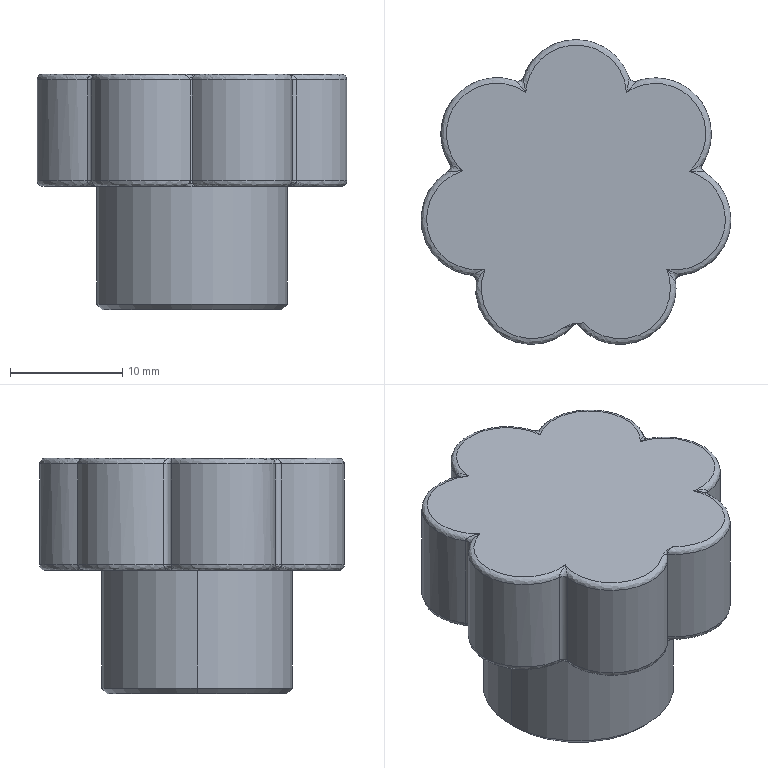Part | SolidWorks | features BaseBody 1 | 1 solid | 61 faces | box 27.635 x 27.19 x 21 mm | volume 7429 mm3 | spline 30 | cylinder 25 | plane 4 | cone 2 | commonest cylinder face diameters 10 x10 1 x9 6 x2 17 x2 22.5 x2